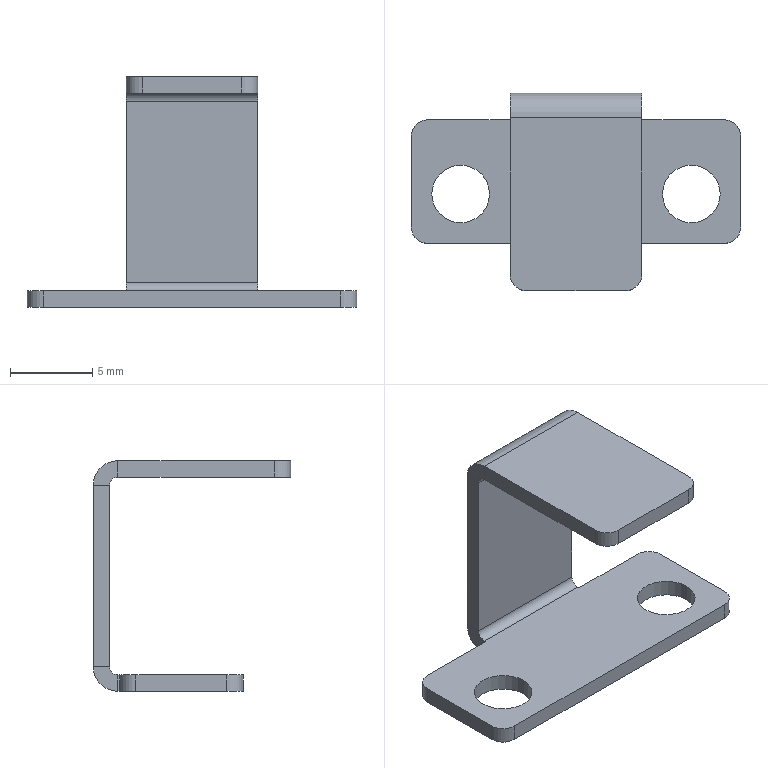Part | SolidWorks | features EdgeFlange 2, BreakCorner 1, FlatPattern 1, SMBaseFlange 1, SheetMetal 1 | 1 solid | 36 faces | box 20 x 12 x 14 mm | volume 327.403 mm3 | plane 22 | cylinder 14 | commonest cylinder face diameters 2 x6 3.5 x4 1 x2 3 x2
STEP:
#1=CARTESIAN_POINT('',(5.25,-0.75,-1.));
#2=VERTEX_POINT('',#1);
#3=CARTESIAN_POINT('',(8.75,-0.75,-1.));
#4=VERTEX_POINT('',#3);
#5=CARTESIAN_POINT('',(7.,-0.75,-1.));
#6=DIRECTION('',(0.,0.,1.));
#7=DIRECTION('',(1.,0.,0.));
#8=AXIS2_PLACEMENT_3D('',#5,#6,#7);
#9=CIRCLE('',#8,1.75);
#10=EDGE_CURVE('',#2,#4,#9,.T.);
#11=ORIENTED_EDGE('',*,*,#10,.F.);
#12=CARTESIAN_POINT('',(5.25,-0.75,0.));
#13=VERTEX_POINT('',#12);
#14=CARTESIAN_POINT('',(5.25,-0.75,-1.));
#15=DIRECTION('',(0.,0.,1.));
#16=VECTOR('',#15,1000.);
#17=LINE('',#14,#16);
#18=EDGE_CURVE('',#2,#13,#17,.T.);
#19=ORIENTED_EDGE('',*,*,#18,.T.);
#20=CARTESIAN_POINT('',(8.75,-0.75,0.));
#21=VERTEX_POINT('',#20);
#22=CARTESIAN_POINT('',(7.,-0.75,0.));
#23=DIRECTION('',(0.,0.,1.));
#24=DIRECTION('',(1.,0.,0.));
#25=AXIS2_PLACEMENT_3D('',#22,#23,#24);
#26=CIRCLE('',#25,1.75);
#27=EDGE_CURVE('',#13,#21,#26,.T.);
#28=ORIENTED_EDGE('',*,*,#27,.T.);
#29=CARTESIAN_POINT('',(8.75,-0.75,-1.));
#30=DIRECTION('',(0.,0.,1.));
#31=VECTOR('',#30,1000.);
#32=LINE('',#29,#31);
#33=EDGE_CURVE('',#4,#21,#32,.T.);
#34=ORIENTED_EDGE('',*,*,#33,.F.);
#35=EDGE_LOOP('',(#11,#19,#28,#34));
#36=FACE_OUTER_BOUND('',#35,.T.);
#37=CARTESIAN_POINT('',(7.,-0.75,-1.));
#38=DIRECTION('',(0.,0.,1.));
#39=DIRECTION('',(1.,0.,0.));
#40=AXIS2_PLACEMENT_3D('',#37,#38,#39);
#41=CYLINDRICAL_SURFACE('',#40,1.75);
#42=ADVANCED_FACE('',(#36),#41,.F.);
#43=CARTESIAN_POINT('',(-8.75,-0.75,-1.));
#44=VERTEX_POINT('',#43);
#45=CARTESIAN_POINT('',(-5.25,-0.75,-1.));
#46=VERTEX_POINT('',#45);
#47=CARTESIAN_POINT('',(-7.,-0.75,-1.));
#48=DIRECTION('',(0.,0.,1.));
#49=DIRECTION('',(1.,0.,0.));
#50=AXIS2_PLACEMENT_3D('',#47,#48,#49);
#51=CIRCLE('',#50,1.75);
#52=EDGE_CURVE('',#44,#46,#51,.T.);
#53=ORIENTED_EDGE('',*,*,#52,.F.);
#54=CARTESIAN_POINT('',(-8.75,-0.75,0.));
#55=VERTEX_POINT('',#54);
#56=CARTESIAN_POINT('',(-8.75,-0.75,-1.));
#57=DIRECTION('',(0.,0.,1.));
#58=VECTOR('',#57,1000.);
#59=LINE('',#56,#58);
#60=EDGE_CURVE('',#44,#55,#59,.T.);
#61=ORIENTED_EDGE('',*,*,#60,.T.);
#62=CARTESIAN_POINT('',(-5.25,-0.75,0.));
#63=VERTEX_POINT('',#62);
#64=CARTESIAN_POINT('',(-7.,-0.75,0.));
#65=DIRECTION('',(0.,0.,1.));
#66=DIRECTION('',(1.,0.,0.));
#67=AXIS2_PLACEMENT_3D('',#64,#65,#66);
#68=CIRCLE('',#67,1.75);
#69=EDGE_CURVE('',#55,#63,#68,.T.);
#70=ORIENTED_EDGE('',*,*,#69,.T.);
#71=CARTESIAN_POINT('',(-5.25,-0.75,-1.));
#72=DIRECTION('',(0.,0.,1.));
#73=VECTOR('',#72,1000.);
#74=LINE('',#71,#73);
#75=EDGE_CURVE('',#46,#63,#74,.T.);
#76=ORIENTED_EDGE('',*,*,#75,.F.);
#77=EDGE_LOOP('',(#53,#61,#70,#76));
#78=FACE_OUTER_BOUND('',#77,.T.);
#79=CARTESIAN_POINT('',(-7.,-0.75,-1.));
#80=DIRECTION('',(0.,0.,1.));
#81=DIRECTION('',(1.,0.,0.));
#82=AXIS2_PLACEMENT_3D('',#79,#80,#81);
#83=CYLINDRICAL_SURFACE('',#82,1.75);
#84=ADVANCED_FACE('',(#78),#83,.F.);
#85=CARTESIAN_POINT('',(4.,4.35,11.5));
#86=VERTEX_POINT('',#85);
#87=CARTESIAN_POINT('',(4.,5.35,11.5));
#88=VERTEX_POINT('',#87);
#89=CARTESIAN_POINT('',(4.,4.35,11.5));
#90=DIRECTION('',(0.,1.,0.));
#91=VECTOR('',#90,1000.);
#92=LINE('',#89,#91);
#93=EDGE_CURVE('',#86,#88,#92,.T.);
#94=ORIENTED_EDGE('',*,*,#93,.F.);
#95=CARTESIAN_POINT('',(4.,4.35,0.5));
#96=VERTEX_POINT('',#95);
#97=CARTESIAN_POINT('',(4.,4.35,0.));
#98=DIRECTION('',(0.,0.,-1.));
#99=VECTOR('',#98,1000.);
#100=LINE('',#97,#99);
#101=EDGE_CURVE('',#86,#96,#100,.T.);
#102=ORIENTED_EDGE('',*,*,#101,.T.);
#103=CARTESIAN_POINT('',(4.,5.35,0.5));
#104=VERTEX_POINT('',#103);
#105=CARTESIAN_POINT('',(4.,5.35,0.5));
#106=DIRECTION('',(0.,1.,0.));
#107=VECTOR('',#106,1000.);
#108=LINE('',#105,#107);
#109=EDGE_CURVE('',#96,#104,#108,.T.);
#110=ORIENTED_EDGE('',*,*,#109,.T.);
#111=CARTESIAN_POINT('',(4.,5.35,0.));
#112=DIRECTION('',(0.,0.,-1.));
#113=VECTOR('',#112,1000.);
#114=LINE('',#111,#113);
#115=EDGE_CURVE('',#88,#104,#114,.T.);
#116=ORIENTED_EDGE('',*,*,#115,.F.);
#117=EDGE_LOOP('',(#94,#102,#110,#116));
#118=FACE_OUTER_BOUND('',#117,.T.);
#119=CARTESIAN_POINT('',(4.,5.35,0.));
#120=DIRECTION('',(-1.,0.,0.));
#121=DIRECTION('',(0.,0.,1.));
#122=AXIS2_PLACEMENT_3D('',#119,#120,#121);
#123=PLANE('',#122);
#124=ADVANCED_FACE('',(#118),#123,.F.);
#125=CARTESIAN_POINT('',(-4.,4.35,11.5));
#126=VERTEX_POINT('',#125);
#127=CARTESIAN_POINT('',(-4.,5.35,11.5));
#128=VERTEX_POINT('',#127);
#129=CARTESIAN_POINT('',(-4.,4.35,11.5));
#130=DIRECTION('',(0.,1.,0.));
#131=VECTOR('',#130,1000.);
#132=LINE('',#129,#131);
#133=EDGE_CURVE('',#126,#128,#132,.T.);
#134=ORIENTED_EDGE('',*,*,#133,.T.);
#135=CARTESIAN_POINT('',(-4.,5.35,0.5));
#136=VERTEX_POINT('',#135);
#137=CARTESIAN_POINT('',(-4.,5.35,0.));
#138=DIRECTION('',(0.,0.,1.));
#139=VECTOR('',#138,1000.);
#140=LINE('',#137,#139);
#141=EDGE_CURVE('',#136,#128,#140,.T.);
#142=ORIENTED_EDGE('',*,*,#141,.F.);
#143=CARTESIAN_POINT('',(-4.,4.35,0.5));
#144=VERTEX_POINT('',#143);
#145=CARTESIAN_POINT('',(-4.,4.35,0.5));
#146=DIRECTION('',(0.,1.,0.));
#147=VECTOR('',#146,1000.);
#148=LINE('',#145,#147);
#149=EDGE_CURVE('',#144,#136,#148,.T.);
#150=ORIENTED_EDGE('',*,*,#149,.F.);
#151=CARTESIAN_POINT('',(-4.,4.35,13.));
#152=DIRECTION('',(0.,0.,1.));
#153=VECTOR('',#152,1000.);
#154=LINE('',#151,#153);
#155=EDGE_CURVE('',#144,#126,#154,.T.);
#156=ORIENTED_EDGE('',*,*,#155,.T.);
#157=EDGE_LOOP('',(#134,#142,#150,#156));
#158=FACE_OUTER_BOUND('',#157,.T.);
#159=CARTESIAN_POINT('',(-4.,5.35,13.));
#160=DIRECTION('',(1.,0.,0.));
#161=DIRECTION('',(0.,0.,-1.));
#162=AXIS2_PLACEMENT_3D('',#159,#160,#161);
#163=PLANE('',#162);
#164=ADVANCED_FACE('',(#158),#163,.F.);
#165=CARTESIAN_POINT('',(-4.,5.35,11.5));
#166=DIRECTION('',(1.,0.,0.));
#167=VECTOR('',#166,1000.);
#168=LINE('',#165,#167);
#169=EDGE_CURVE('',#128,#88,#168,.T.);
#170=ORIENTED_EDGE('',*,*,#169,.T.);
#171=ORIENTED_EDGE('',*,*,#115,.T.);
#172=CARTESIAN_POINT('',(4.,5.35,0.5));
#173=DIRECTION('',(1.,0.,0.));
#174=VECTOR('',#173,1000.);
#175=LINE('',#172,#174);
#176=EDGE_CURVE('',#136,#104,#175,.T.);
#177=ORIENTED_EDGE('',*,*,#176,.F.);
#178=ORIENTED_EDGE('',*,*,#141,.T.);
#179=EDGE_LOOP('',(#170,#171,#177,#178));
#180=FACE_OUTER_BOUND('',#179,.T.);
#181=CARTESIAN_POINT('',(0.,5.35,0.));
#182=DIRECTION('',(0.,-1.,0.));
#183=DIRECTION('',(0.,0.,-1.));
#184=AXIS2_PLACEMENT_3D('',#181,#182,#183);
#185=PLANE('',#184);
#186=ADVANCED_FACE('',(#180),#185,.F.);
#187=ORIENTED_EDGE('',*,*,#101,.F.);
#188=CARTESIAN_POINT('',(-4.,4.35,11.5));
#189=DIRECTION('',(1.,0.,0.));
#190=VECTOR('',#189,1000.);
#191=LINE('',#188,#190);
#192=EDGE_CURVE('',#126,#86,#191,.T.);
#193=ORIENTED_EDGE('',*,*,#192,.F.);
#194=ORIENTED_EDGE('',*,*,#155,.F.);
#195=CARTESIAN_POINT('',(4.,4.35,0.5));
#196=DIRECTION('',(-1.,0.,0.));
#197=VECTOR('',#196,1000.);
#198=LINE('',#195,#197);
#199=EDGE_CURVE('',#96,#144,#198,.T.);
#200=ORIENTED_EDGE('',*,*,#199,.F.);
#201=EDGE_LOOP('',(#187,#193,#194,#200));
#202=FACE_OUTER_BOUND('',#201,.T.);
#203=CARTESIAN_POINT('',(0.,4.35,0.));
#204=DIRECTION('',(0.,-1.,0.));
#205=DIRECTION('',(0.,0.,-1.));
#206=AXIS2_PLACEMENT_3D('',#203,#204,#205);
#207=PLANE('',#206);
#208=ADVANCED_FACE('',(#202),#207,.T.);
#209=CARTESIAN_POINT('',(-4.,3.75,-1.));
#210=VERTEX_POINT('',#209);
#211=CARTESIAN_POINT('',(-9.,3.75,-1.));
#212=VERTEX_POINT('',#211);
#213=CARTESIAN_POINT('',(-10.,3.75,-1.));
#214=DIRECTION('',(-1.,0.,0.));
#215=VECTOR('',#214,1000.);
#216=LINE('',#213,#215);
#217=EDGE_CURVE('',#210,#212,#216,.T.);
#218=ORIENTED_EDGE('',*,*,#217,.T.);
#219=CARTESIAN_POINT('',(-9.,3.75,0.));
#220=VERTEX_POINT('',#219);
#221=CARTESIAN_POINT('',(-9.,3.75,-1.));
#222=DIRECTION('',(0.,0.,1.));
#223=VECTOR('',#222,1000.);
#224=LINE('',#221,#223);
#225=EDGE_CURVE('',#212,#220,#224,.T.);
#226=ORIENTED_EDGE('',*,*,#225,.T.);
#227=CARTESIAN_POINT('',(-4.,3.75,0.));
#228=VERTEX_POINT('',#227);
#229=CARTESIAN_POINT('',(-10.,3.75,0.));
#230=DIRECTION('',(-1.,0.,0.));
#231=VECTOR('',#230,1000.);
#232=LINE('',#229,#231);
#233=EDGE_CURVE('',#228,#220,#232,.T.);
#234=ORIENTED_EDGE('',*,*,#233,.F.);
#235=CARTESIAN_POINT('',(-4.,3.75,0.));
#236=DIRECTION('',(0.,0.,-1.));
#237=VECTOR('',#236,1000.);
#238=LINE('',#235,#237);
#239=EDGE_CURVE('',#228,#210,#238,.T.);
#240=ORIENTED_EDGE('',*,*,#239,.T.);
#241=EDGE_LOOP('',(#218,#226,#234,#240));
#242=FACE_OUTER_BOUND('',#241,.T.);
#243=CARTESIAN_POINT('',(-10.,3.75,-1.));
#244=DIRECTION('',(0.,1.,0.));
#245=DIRECTION('',(0.,0.,1.));
#246=AXIS2_PLACEMENT_3D('',#243,#244,#245);
#247=PLANE('',#246);
#248=ADVANCED_FACE('',(#242),#247,.T.);
#249=CARTESIAN_POINT('',(10.,-2.75,0.));
#250=VERTEX_POINT('',#249);
#251=CARTESIAN_POINT('',(10.,2.75,0.));
#252=VERTEX_POINT('',#251);
#253=CARTESIAN_POINT('',(10.,-3.75,0.));
#254=DIRECTION('',(0.,1.,0.));
#255=VECTOR('',#254,1000.);
#256=LINE('',#253,#255);
#257=EDGE_CURVE('',#250,#252,#256,.T.);
#258=ORIENTED_EDGE('',*,*,#257,.F.);
#259=CARTESIAN_POINT('',(10.,-2.75,-1.));
#260=VERTEX_POINT('',#259);
#261=CARTESIAN_POINT('',(10.,-2.75,-1.));
#262=DIRECTION('',(0.,0.,-1.));
#263=VECTOR('',#262,1000.);
#264=LINE('',#261,#263);
#265=EDGE_CURVE('',#250,#260,#264,.T.);
#266=ORIENTED_EDGE('',*,*,#265,.T.);
#267=CARTESIAN_POINT('',(10.,2.75,-1.));
#268=VERTEX_POINT('',#267);
#269=CARTESIAN_POINT('',(10.,-3.75,-1.));
#270=DIRECTION('',(0.,1.,0.));
#271=VECTOR('',#270,1000.);
#272=LINE('',#269,#271);
#273=EDGE_CURVE('',#260,#268,#272,.T.);
#274=ORIENTED_EDGE('',*,*,#273,.T.);
#275=CARTESIAN_POINT('',(10.,2.75,-1.));
#276=DIRECTION('',(0.,0.,1.));
#277=VECTOR('',#276,1000.);
#278=LINE('',#275,#277);
#279=EDGE_CURVE('',#268,#252,#278,.T.);
#280=ORIENTED_EDGE('',*,*,#279,.T.);
#281=EDGE_LOOP('',(#258,#266,#274,#280));
#282=FACE_OUTER_BOUND('',#281,.T.);
#283=CARTESIAN_POINT('',(10.,-3.75,-1.));
#284=DIRECTION('',(1.,0.,0.));
#285=DIRECTION('',(0.,0.,-1.));
#286=AXIS2_PLACEMENT_3D('',#283,#284,#285);
#287=PLANE('',#286);
#288=ADVANCED_FACE('',(#282),#287,.T.);
#289=CARTESIAN_POINT('',(-9.,-3.75,-1.));
#290=VERTEX_POINT('',#289);
#291=CARTESIAN_POINT('',(9.,-3.75,-1.));
#292=VERTEX_POINT('',#291);
#293=CARTESIAN_POINT('',(-10.,-3.75,-1.));
#294=DIRECTION('',(1.,0.,0.));
#295=VECTOR('',#294,1000.);
#296=LINE('',#293,#295);
#297=EDGE_CURVE('',#290,#292,#296,.T.);
#298=ORIENTED_EDGE('',*,*,#297,.T.);
#299=CARTESIAN_POINT('',(9.,-3.75,0.));
#300=VERTEX_POINT('',#299);
#301=CARTESIAN_POINT('',(9.,-3.75,-1.));
#302=DIRECTION('',(0.,0.,1.));
#303=VECTOR('',#302,1000.);
#304=LINE('',#301,#303);
#305=EDGE_CURVE('',#292,#300,#304,.T.);
#306=ORIENTED_EDGE('',*,*,#305,.T.);
#307=CARTESIAN_POINT('',(-9.,-3.75,0.));
#308=VERTEX_POINT('',#307);
#309=CARTESIAN_POINT('',(-10.,-3.75,0.));
#310=DIRECTION('',(1.,0.,0.));
#311=VECTOR('',#310,1000.);
#312=LINE('',#309,#311);
#313=EDGE_CURVE('',#308,#300,#312,.T.);
#314=ORIENTED_EDGE('',*,*,#313,.F.);
#315=CARTESIAN_POINT('',(-9.,-3.75,-1.));
#316=DIRECTION('',(0.,0.,-1.));
#317=VECTOR('',#316,1000.);
#318=LINE('',#315,#317);
#319=EDGE_CURVE('',#308,#290,#318,.T.);
#320=ORIENTED_EDGE('',*,*,#319,.T.);
#321=EDGE_LOOP('',(#298,#306,#314,#320));
#322=FACE_OUTER_BOUND('',#321,.T.);
#323=CARTESIAN_POINT('',(-10.,-3.75,-1.));
#324=DIRECTION('',(0.,-1.,0.));
#325=DIRECTION('',(0.,0.,-1.));
#326=AXIS2_PLACEMENT_3D('',#323,#324,#325);
#327=PLANE('',#326);
#328=ADVANCED_FACE('',(#322),#327,.T.);
#329=CARTESIAN_POINT('',(-10.,2.75,-1.));
#330=VERTEX_POINT('',#329);
#331=CARTESIAN_POINT('',(-10.,-2.75,-1.));
#332=VERTEX_POINT('',#331);
#333=CARTESIAN_POINT('',(-10.,-3.75,-1.));
#334=DIRECTION('',(0.,-1.,0.));
#335=VECTOR('',#334,1000.);
#336=LINE('',#333,#335);
#337=EDGE_CURVE('',#330,#332,#336,.T.);
#338=ORIENTED_EDGE('',*,*,#337,.T.);
#339=CARTESIAN_POINT('',(-10.,-2.75,0.));
#340=VERTEX_POINT('',#339);
#341=CARTESIAN_POINT('',(-10.,-2.75,-1.));
#342=DIRECTION('',(0.,0.,1.));
#343=VECTOR('',#342,1000.);
#344=LINE('',#341,#343);
#345=EDGE_CURVE('',#332,#340,#344,.T.);
#346=ORIENTED_EDGE('',*,*,#345,.T.);
#347=CARTESIAN_POINT('',(-10.,2.75,0.));
#348=VERTEX_POINT('',#347);
#349=CARTESIAN_POINT('',(-10.,-3.75,0.));
#350=DIRECTION('',(0.,-1.,0.));
#351=VECTOR('',#350,1000.);
#352=LINE('',#349,#351);
#353=EDGE_CURVE('',#348,#340,#352,.T.);
#354=ORIENTED_EDGE('',*,*,#353,.F.);
#355=CARTESIAN_POINT('',(-10.,2.75,-1.));
#356=DIRECTION('',(0.,0.,-1.));
#357=VECTOR('',#356,1000.);
#358=LINE('',#355,#357);
#359=EDGE_CURVE('',#348,#330,#358,.T.);
#360=ORIENTED_EDGE('',*,*,#359,.T.);
#361=EDGE_LOOP('',(#338,#346,#354,#360));
#362=FACE_OUTER_BOUND('',#361,.T.);
#363=CARTESIAN_POINT('',(-10.,-3.75,-1.));
#364=DIRECTION('',(-1.,0.,0.));
#365=DIRECTION('',(0.,0.,1.));
#366=AXIS2_PLACEMENT_3D('',#363,#364,#365);
#367=PLANE('',#366);
#368=ADVANCED_FACE('',(#362),#367,.T.);
#369=CARTESIAN_POINT('',(9.,3.75,0.));
#370=VERTEX_POINT('',#369);
#371=CARTESIAN_POINT('',(4.,3.75,0.));
#372=VERTEX_POINT('',#371);
#373=CARTESIAN_POINT('',(-10.,3.75,0.));
#374=DIRECTION('',(-1.,0.,0.));
#375=VECTOR('',#374,1000.);
#376=LINE('',#373,#375);
#377=EDGE_CURVE('',#370,#372,#376,.T.);
#378=ORIENTED_EDGE('',*,*,#377,.F.);
#379=CARTESIAN_POINT('',(9.,3.75,-1.));
#380=VERTEX_POINT('',#379);
#381=CARTESIAN_POINT('',(9.,3.75,-1.));
#382=DIRECTION('',(0.,0.,-1.));
#383=VECTOR('',#382,1000.);
#384=LINE('',#381,#383);
#385=EDGE_CURVE('',#370,#380,#384,.T.);
#386=ORIENTED_EDGE('',*,*,#385,.T.);
#387=CARTESIAN_POINT('',(4.,3.75,-1.));
#388=VERTEX_POINT('',#387);
#389=CARTESIAN_POINT('',(-10.,3.75,-1.));
#390=DIRECTION('',(-1.,0.,0.));
#391=VECTOR('',#390,1000.);
#392=LINE('',#389,#391);
#393=EDGE_CURVE('',#380,#388,#392,.T.);
#394=ORIENTED_EDGE('',*,*,#393,.T.);
#395=CARTESIAN_POINT('',(4.,3.75,0.));
#396=DIRECTION('',(0.,0.,-1.));
#397=VECTOR('',#396,1000.);
#398=LINE('',#395,#397);
#399=EDGE_CURVE('',#372,#388,#398,.T.);
#400=ORIENTED_EDGE('',*,*,#399,.F.);
#401=EDGE_LOOP('',(#378,#386,#394,#400));
#402=FACE_OUTER_BOUND('',#401,.T.);
#403=CARTESIAN_POINT('',(-10.,3.75,-1.));
#404=DIRECTION('',(0.,1.,0.));
#405=DIRECTION('',(0.,0.,1.));
#406=AXIS2_PLACEMENT_3D('',#403,#404,#405);
#407=PLANE('',#406);
#408=ADVANCED_FACE('',(#402),#407,.T.);
#409=CARTESIAN_POINT('',(7.,-0.75,-1.));
#410=DIRECTION('',(0.,0.,1.));
#411=DIRECTION('',(1.,0.,0.));
#412=AXIS2_PLACEMENT_3D('',#409,#410,#411);
#413=CIRCLE('',#412,1.75);
#414=EDGE_CURVE('',#4,#2,#413,.T.);
#415=ORIENTED_EDGE('',*,*,#414,.T.);
#416=ORIENTED_EDGE('',*,*,#10,.T.);
#417=EDGE_LOOP('',(#415,#416));
#418=FACE_BOUND('',#417,.T.);
#419=CARTESIAN_POINT('',(-7.,-0.75,-1.));
#420=DIRECTION('',(0.,0.,1.));
#421=DIRECTION('',(1.,0.,0.));
#422=AXIS2_PLACEMENT_3D('',#419,#420,#421);
#423=CIRCLE('',#422,1.75);
#424=EDGE_CURVE('',#46,#44,#423,.T.);
#425=ORIENTED_EDGE('',*,*,#424,.T.);
#426=ORIENTED_EDGE('',*,*,#52,.T.);
#427=EDGE_LOOP('',(#425,#426));
#428=FACE_BOUND('',#427,.T.);
#429=ORIENTED_EDGE('',*,*,#273,.F.);
#430=CARTESIAN_POINT('',(9.,-2.75,-1.));
#431=DIRECTION('',(0.,0.,-1.));
#432=DIRECTION('',(-1.,0.,0.));
#433=AXIS2_PLACEMENT_3D('',#430,#431,#432);
#434=CIRCLE('',#433,1.);
#435=EDGE_CURVE('',#260,#292,#434,.T.);
#436=ORIENTED_EDGE('',*,*,#435,.T.);
#437=ORIENTED_EDGE('',*,*,#297,.F.);
#438=CARTESIAN_POINT('',(-9.,-2.75,-1.));
#439=DIRECTION('',(0.,0.,-1.));
#440=DIRECTION('',(-1.,0.,0.));
#441=AXIS2_PLACEMENT_3D('',#438,#439,#440);
#442=CIRCLE('',#441,1.);
#443=EDGE_CURVE('',#290,#332,#442,.T.);
#444=ORIENTED_EDGE('',*,*,#443,.T.);
#445=ORIENTED_EDGE('',*,*,#337,.F.);
#446=CARTESIAN_POINT('',(-9.,2.75,-1.));
#447=DIRECTION('',(0.,0.,-1.));
#448=DIRECTION('',(-1.,0.,0.));
#449=AXIS2_PLACEMENT_3D('',#446,#447,#448);
#450=CIRCLE('',#449,1.);
#451=EDGE_CURVE('',#330,#212,#450,.T.);
#452=ORIENTED_EDGE('',*,*,#451,.T.);
#453=ORIENTED_EDGE('',*,*,#217,.F.);
#454=CARTESIAN_POINT('',(-4.,3.85,-1.));
#455=VERTEX_POINT('',#454);
#456=CARTESIAN_POINT('',(-4.,3.85,-1.));
#457=DIRECTION('',(0.,-1.,0.));
#458=VECTOR('',#457,1000.);
#459=LINE('',#456,#458);
#460=EDGE_CURVE('',#455,#210,#459,.T.);
#461=ORIENTED_EDGE('',*,*,#460,.F.);
#462=CARTESIAN_POINT('',(4.,3.85,-1.));
#463=VERTEX_POINT('',#462);
#464=CARTESIAN_POINT('',(-4.,3.85,-1.));
#465=DIRECTION('',(1.,0.,0.));
#466=VECTOR('',#465,1000.);
#467=LINE('',#464,#466);
#468=EDGE_CURVE('',#455,#463,#467,.T.);
#469=ORIENTED_EDGE('',*,*,#468,.T.);
#470=CARTESIAN_POINT('',(4.,3.85,-1.));
#471=DIRECTION('',(0.,-1.,0.));
#472=VECTOR('',#471,1000.);
#473=LINE('',#470,#472);
#474=EDGE_CURVE('',#463,#388,#473,.T.);
#475=ORIENTED_EDGE('',*,*,#474,.T.);
#476=ORIENTED_EDGE('',*,*,#393,.F.);
#477=CARTESIAN_POINT('',(9.,2.75,-1.));
#478=DIRECTION('',(0.,0.,-1.));
#479=DIRECTION('',(-1.,0.,0.));
#480=AXIS2_PLACEMENT_3D('',#477,#478,#479);
#481=CIRCLE('',#480,1.);
#482=EDGE_CURVE('',#380,#268,#481,.T.);
#483=ORIENTED_EDGE('',*,*,#482,.T.);
#484=EDGE_LOOP('',(#429,#436,#437,#444,#445,#452,#453,#461,#469,#475,#476,#483));
#485=FACE_OUTER_BOUND('',#484,.T.);
#486=CARTESIAN_POINT('',(0.,0.,-1.));
#487=DIRECTION('',(0.,0.,-1.));
#488=DIRECTION('',(-1.,0.,0.));
#489=AXIS2_PLACEMENT_3D('',#486,#487,#488);
#490=PLANE('',#489);
#491=ADVANCED_FACE('',(#418,#428,#485),#490,.T.);
#492=CARTESIAN_POINT('',(7.,-0.75,0.));
#493=DIRECTION('',(0.,0.,1.));
#494=DIRECTION('',(1.,0.,0.));
#495=AXIS2_PLACEMENT_3D('',#492,#493,#494);
#496=CIRCLE('',#495,1.75);
#497=EDGE_CURVE('',#21,#13,#496,.T.);
#498=ORIENTED_EDGE('',*,*,#497,.F.);
#499=ORIENTED_EDGE('',*,*,#27,.F.);
#500=EDGE_LOOP('',(#498,#499));
#501=FACE_BOUND('',#500,.T.);
#502=CARTESIAN_POINT('',(-7.,-0.75,0.));
#503=DIRECTION('',(0.,0.,1.));
#504=DIRECTION('',(1.,0.,0.));
#505=AXIS2_PLACEMENT_3D('',#502,#503,#504);
#506=CIRCLE('',#505,1.75);
#507=EDGE_CURVE('',#63,#55,#506,.T.);
#508=ORIENTED_EDGE('',*,*,#507,.F.);
#509=ORIENTED_EDGE('',*,*,#69,.F.);
#510=EDGE_LOOP('',(#508,#509));
#511=FACE_BOUND('',#510,.T.);
#512=ORIENTED_EDGE('',*,*,#313,.T.);
#513=CARTESIAN_POINT('',(9.,-2.75,0.));
#514=DIRECTION('',(0.,0.,1.));
#515=DIRECTION('',(-1.,0.,0.));
#516=AXIS2_PLACEMENT_3D('',#513,#514,#515);
#517=CIRCLE('',#516,1.);
#518=EDGE_CURVE('',#300,#250,#517,.T.);
#519=ORIENTED_EDGE('',*,*,#518,.T.);
#520=ORIENTED_EDGE('',*,*,#257,.T.);
#521=CARTESIAN_POINT('',(9.,2.75,0.));
#522=DIRECTION('',(0.,0.,1.));
#523=DIRECTION('',(-1.,0.,0.));
#524=AXIS2_PLACEMENT_3D('',#521,#522,#523);
#525=CIRCLE('',#524,1.);
#526=EDGE_CURVE('',#252,#370,#525,.T.);
#527=ORIENTED_EDGE('',*,*,#526,.T.);
#528=ORIENTED_EDGE('',*,*,#377,.T.);
#529=CARTESIAN_POINT('',(4.,3.85,0.));
#530=VERTEX_POINT('',#529);
#531=CARTESIAN_POINT('',(4.,3.85,0.));
#532=DIRECTION('',(0.,-1.,0.));
#533=VECTOR('',#532,1000.);
#534=LINE('',#531,#533);
#535=EDGE_CURVE('',#530,#372,#534,.T.);
#536=ORIENTED_EDGE('',*,*,#535,.F.);
#537=CARTESIAN_POINT('',(-4.,3.85,0.));
#538=VERTEX_POINT('',#537);
#539=CARTESIAN_POINT('',(-4.,3.85,0.));
#540=DIRECTION('',(1.,0.,0.));
#541=VECTOR('',#540,1000.);
#542=LINE('',#539,#541);
#543=EDGE_CURVE('',#538,#530,#542,.T.);
#544=ORIENTED_EDGE('',*,*,#543,.F.);
#545=CARTESIAN_POINT('',(-4.,3.85,0.));
#546=DIRECTION('',(0.,-1.,0.));
#547=VECTOR('',#546,1000.);
#548=LINE('',#545,#547);
#549=EDGE_CURVE('',#538,#228,#548,.T.);
#550=ORIENTED_EDGE('',*,*,#549,.T.);
#551=ORIENTED_EDGE('',*,*,#233,.T.);
#552=CARTESIAN_POINT('',(-9.,2.75,0.));
#553=DIRECTION('',(0.,0.,1.));
#554=DIRECTION('',(-1.,0.,0.));
#555=AXIS2_PLACEMENT_3D('',#552,#553,#554);
#556=CIRCLE('',#555,1.);
#557=EDGE_CURVE('',#220,#348,#556,.T.);
#558=ORIENTED_EDGE('',*,*,#557,.T.);
#559=ORIENTED_EDGE('',*,*,#353,.T.);
#560=CARTESIAN_POINT('',(-9.,-2.75,0.));
#561=DIRECTION('',(0.,0.,1.));
#562=DIRECTION('',(-1.,0.,0.));
#563=AXIS2_PLACEMENT_3D('',#560,#561,#562);
#564=CIRCLE('',#563,1.);
#565=EDGE_CURVE('',#340,#308,#564,.T.);
#566=ORIENTED_EDGE('',*,*,#565,.T.);
#567=EDGE_LOOP('',(#512,#519,#520,#527,#528,#536,#544,#550,#551,#558,#559,#566));
#568=FACE_OUTER_BOUND('',#567,.T.);
#569=CARTESIAN_POINT('',(0.,0.,0.));
#570=DIRECTION('',(0.,0.,-1.));
#571=DIRECTION('',(-1.,0.,0.));
#572=AXIS2_PLACEMENT_3D('',#569,#570,#571);
#573=PLANE('',#572);
#574=ADVANCED_FACE('',(#501,#511,#568),#573,.F.);
#575=ORIENTED_EDGE('',*,*,#60,.F.);
#576=ORIENTED_EDGE('',*,*,#424,.F.);
#577=ORIENTED_EDGE('',*,*,#75,.T.);
#578=ORIENTED_EDGE('',*,*,#507,.T.);
#579=EDGE_LOOP('',(#575,#576,#577,#578));
#580=FACE_OUTER_BOUND('',#579,.T.);
#581=CARTESIAN_POINT('',(-7.,-0.75,-1.));
#582=DIRECTION('',(0.,0.,1.));
#583=DIRECTION('',(1.,0.,0.));
#584=AXIS2_PLACEMENT_3D('',#581,#582,#583);
#585=CYLINDRICAL_SURFACE('',#584,1.75);
#586=ADVANCED_FACE('',(#580),#585,.F.);
#587=ORIENTED_EDGE('',*,*,#18,.F.);
#588=ORIENTED_EDGE('',*,*,#414,.F.);
#589=ORIENTED_EDGE('',*,*,#33,.T.);
#590=ORIENTED_EDGE('',*,*,#497,.T.);
#591=EDGE_LOOP('',(#587,#588,#589,#590));
#592=FACE_OUTER_BOUND('',#591,.T.);
#593=CARTESIAN_POINT('',(7.,-0.75,-1.));
#594=DIRECTION('',(0.,0.,1.));
#595=DIRECTION('',(1.,0.,0.));
#596=AXIS2_PLACEMENT_3D('',#593,#594,#595);
#597=CYLINDRICAL_SURFACE('',#596,1.75);
#598=ADVANCED_FACE('',(#592),#597,.F.);
#599=ORIENTED_EDGE('',*,*,#549,.F.);
#600=CARTESIAN_POINT('',(-4.,3.85,0.));
#601=DIRECTION('',(0.,0.,-1.));
#602=VECTOR('',#601,1000.);
#603=LINE('',#600,#602);
#604=EDGE_CURVE('',#538,#455,#603,.T.);
#605=ORIENTED_EDGE('',*,*,#604,.T.);
#606=ORIENTED_EDGE('',*,*,#460,.T.);
#607=ORIENTED_EDGE('',*,*,#239,.F.);
#608=EDGE_LOOP('',(#599,#605,#606,#607));
#609=FACE_OUTER_BOUND('',#608,.T.);
#610=CARTESIAN_POINT('',(-4.,3.85,0.));
#611=DIRECTION('',(-1.,0.,0.));
#612=DIRECTION('',(0.,0.,-1.));
#613=AXIS2_PLACEMENT_3D('',#610,#611,#612);
#614=PLANE('',#613);
#615=ADVANCED_FACE('',(#609),#614,.T.);
#616=ORIENTED_EDGE('',*,*,#474,.F.);
#617=CARTESIAN_POINT('',(4.,3.85,0.));
#618=DIRECTION('',(0.,0.,-1.));
#619=VECTOR('',#618,1000.);
#620=LINE('',#617,#619);
#621=EDGE_CURVE('',#530,#463,#620,.T.);
#622=ORIENTED_EDGE('',*,*,#621,.F.);
#623=ORIENTED_EDGE('',*,*,#535,.T.);
#624=ORIENTED_EDGE('',*,*,#399,.T.);
#625=EDGE_LOOP('',(#616,#622,#623,#624));
#626=FACE_OUTER_BOUND('',#625,.T.);
#627=CARTESIAN_POINT('',(4.,3.85,0.));
#628=DIRECTION('',(-1.,0.,0.));
#629=DIRECTION('',(0.,0.,-1.));
#630=AXIS2_PLACEMENT_3D('',#627,#628,#629);
#631=PLANE('',#630);
#632=ADVANCED_FACE('',(#626),#631,.F.);
#633=ORIENTED_EDGE('',*,*,#109,.F.);
#634=CARTESIAN_POINT('',(4.,3.85,0.5));
#635=DIRECTION('',(1.,0.,0.));
#636=DIRECTION('',(0.,0.,1.));
#637=AXIS2_PLACEMENT_3D('',#634,#635,#636);
#638=CIRCLE('',#637,0.5);
#639=EDGE_CURVE('',#530,#96,#638,.T.);
#640=ORIENTED_EDGE('',*,*,#639,.F.);
#641=ORIENTED_EDGE('',*,*,#621,.T.);
#642=CARTESIAN_POINT('',(4.,3.85,0.5));
#643=DIRECTION('',(1.,0.,0.));
#644=DIRECTION('',(0.,0.,1.));
#645=AXIS2_PLACEMENT_3D('',#642,#643,#644);
#646=CIRCLE('',#645,1.5);
#647=EDGE_CURVE('',#463,#104,#646,.T.);
#648=ORIENTED_EDGE('',*,*,#647,.T.);
#649=EDGE_LOOP('',(#633,#640,#641,#648));
#650=FACE_OUTER_BOUND('',#649,.T.);
#651=CARTESIAN_POINT('',(4.,3.85,0.5));
#652=DIRECTION('',(1.,0.,0.));
#653=DIRECTION('',(0.,0.,-1.));
#654=AXIS2_PLACEMENT_3D('',#651,#652,#653);
#655=PLANE('',#654);
#656=ADVANCED_FACE('',(#650),#655,.T.);
#657=CARTESIAN_POINT('',(-4.,3.85,0.5));
#658=DIRECTION('',(-1.,0.,0.));
#659=DIRECTION('',(0.,0.,1.));
#660=AXIS2_PLACEMENT_3D('',#657,#658,#659);
#661=CIRCLE('',#660,0.5);
#662=EDGE_CURVE('',#144,#538,#661,.T.);
#663=ORIENTED_EDGE('',*,*,#662,.F.);
#664=ORIENTED_EDGE('',*,*,#149,.T.);
#665=CARTESIAN_POINT('',(-4.,3.85,0.5));
#666=DIRECTION('',(-1.,0.,0.));
#667=DIRECTION('',(0.,0.,1.));
#668=AXIS2_PLACEMENT_3D('',#665,#666,#667);
#669=CIRCLE('',#668,1.5);
#670=EDGE_CURVE('',#136,#455,#669,.T.);
#671=ORIENTED_EDGE('',*,*,#670,.T.);
#672=ORIENTED_EDGE('',*,*,#604,.F.);
#673=EDGE_LOOP('',(#663,#664,#671,#672));
#674=FACE_OUTER_BOUND('',#673,.T.);
#675=CARTESIAN_POINT('',(-4.,3.85,0.5));
#676=DIRECTION('',(1.,0.,0.));
#677=DIRECTION('',(0.,0.,-1.));
#678=AXIS2_PLACEMENT_3D('',#675,#676,#677);
#679=PLANE('',#678);
#680=ADVANCED_FACE('',(#674),#679,.F.);
#681=ORIENTED_EDGE('',*,*,#468,.F.);
#682=ORIENTED_EDGE('',*,*,#670,.F.);
#683=ORIENTED_EDGE('',*,*,#176,.T.);
#684=ORIENTED_EDGE('',*,*,#647,.F.);
#685=EDGE_LOOP('',(#681,#682,#683,#684));
#686=FACE_OUTER_BOUND('',#685,.T.);
#687=CARTESIAN_POINT('',(-4.,3.85,0.5));
#688=DIRECTION('',(-1.,0.,0.));
#689=DIRECTION('',(0.,1.,0.));
#690=AXIS2_PLACEMENT_3D('',#687,#688,#689);
#691=CYLINDRICAL_SURFACE('',#690,1.5);
#692=ADVANCED_FACE('',(#686),#691,.T.);
#693=ORIENTED_EDGE('',*,*,#543,.T.);
#694=ORIENTED_EDGE('',*,*,#639,.T.);
#695=ORIENTED_EDGE('',*,*,#199,.T.);
#696=ORIENTED_EDGE('',*,*,#662,.T.);
#697=EDGE_LOOP('',(#693,#694,#695,#696));
#698=FACE_OUTER_BOUND('',#697,.T.);
#699=CARTESIAN_POINT('',(-4.,3.85,0.5));
#700=DIRECTION('',(-1.,0.,0.));
#701=DIRECTION('',(0.,1.,0.));
#702=AXIS2_PLACEMENT_3D('',#699,#700,#701);
#703=CYLINDRICAL_SURFACE('',#702,0.5);
#704=ADVANCED_FACE('',(#698),#703,.F.);
#705=CARTESIAN_POINT('',(4.,3.85,12.));
#706=VERTEX_POINT('',#705);
#707=CARTESIAN_POINT('',(4.,3.85,13.));
#708=VERTEX_POINT('',#707);
#709=CARTESIAN_POINT('',(4.,3.85,13.));
#710=DIRECTION('',(0.,0.,1.));
#711=VECTOR('',#710,1000.);
#712=LINE('',#709,#711);
#713=EDGE_CURVE('',#706,#708,#712,.T.);
#714=ORIENTED_EDGE('',*,*,#713,.F.);
#715=CARTESIAN_POINT('',(4.,3.85,11.5));
#716=DIRECTION('',(1.,0.,0.));
#717=DIRECTION('',(0.,0.,1.));
#718=AXIS2_PLACEMENT_3D('',#715,#716,#717);
#719=CIRCLE('',#718,0.5);
#720=EDGE_CURVE('',#86,#706,#719,.T.);
#721=ORIENTED_EDGE('',*,*,#720,.F.);
#722=ORIENTED_EDGE('',*,*,#93,.T.);
#723=CARTESIAN_POINT('',(4.,3.85,11.5));
#724=DIRECTION('',(1.,0.,0.));
#725=DIRECTION('',(0.,0.,1.));
#726=AXIS2_PLACEMENT_3D('',#723,#724,#725);
#727=CIRCLE('',#726,1.5);
#728=EDGE_CURVE('',#88,#708,#727,.T.);
#729=ORIENTED_EDGE('',*,*,#728,.T.);
#730=EDGE_LOOP('',(#714,#721,#722,#729));
#731=FACE_OUTER_BOUND('',#730,.T.);
#732=CARTESIAN_POINT('',(4.,3.85,11.5));
#733=DIRECTION('',(1.,0.,0.));
#734=DIRECTION('',(0.,0.,-1.));
#735=AXIS2_PLACEMENT_3D('',#732,#733,#734);
#736=PLANE('',#735);
#737=ADVANCED_FACE('',(#731),#736,.T.);
#738=CARTESIAN_POINT('',(-4.,3.85,12.));
#739=VERTEX_POINT('',#738);
#740=CARTESIAN_POINT('',(-4.,3.85,11.5));
#741=DIRECTION('',(-1.,0.,0.));
#742=DIRECTION('',(0.,0.,1.));
#743=AXIS2_PLACEMENT_3D('',#740,#741,#742);
#744=CIRCLE('',#743,0.5);
#745=EDGE_CURVE('',#739,#126,#744,.T.);
#746=ORIENTED_EDGE('',*,*,#745,.F.);
#747=CARTESIAN_POINT('',(-4.,3.85,13.));
#748=VERTEX_POINT('',#747);
#749=CARTESIAN_POINT('',(-4.,3.85,12.));
#750=DIRECTION('',(0.,0.,1.));
#751=VECTOR('',#750,1000.);
#752=LINE('',#749,#751);
#753=EDGE_CURVE('',#739,#748,#752,.T.);
#754=ORIENTED_EDGE('',*,*,#753,.T.);
#755=CARTESIAN_POINT('',(-4.,3.85,11.5));
#756=DIRECTION('',(-1.,0.,0.));
#757=DIRECTION('',(0.,0.,1.));
#758=AXIS2_PLACEMENT_3D('',#755,#756,#757);
#759=CIRCLE('',#758,1.5);
#760=EDGE_CURVE('',#748,#128,#759,.T.);
#761=ORIENTED_EDGE('',*,*,#760,.T.);
#762=ORIENTED_EDGE('',*,*,#133,.F.);
#763=EDGE_LOOP('',(#746,#754,#761,#762));
#764=FACE_OUTER_BOUND('',#763,.T.);
#765=CARTESIAN_POINT('',(-4.,3.85,11.5));
#766=DIRECTION('',(1.,0.,0.));
#767=DIRECTION('',(0.,0.,-1.));
#768=AXIS2_PLACEMENT_3D('',#765,#766,#767);
#769=PLANE('',#768);
#770=ADVANCED_FACE('',(#764),#769,.F.);
#771=ORIENTED_EDGE('',*,*,#169,.F.);
#772=ORIENTED_EDGE('',*,*,#760,.F.);
#773=CARTESIAN_POINT('',(4.,3.85,13.));
#774=DIRECTION('',(1.,0.,0.));
#775=VECTOR('',#774,1000.);
#776=LINE('',#773,#775);
#777=EDGE_CURVE('',#748,#708,#776,.T.);
#778=ORIENTED_EDGE('',*,*,#777,.T.);
#779=ORIENTED_EDGE('',*,*,#728,.F.);
#780=EDGE_LOOP('',(#771,#772,#778,#779));
#781=FACE_OUTER_BOUND('',#780,.T.);
#782=CARTESIAN_POINT('',(-4.,3.85,11.5));
#783=DIRECTION('',(-1.,0.,0.));
#784=DIRECTION('',(0.,0.,1.));
#785=AXIS2_PLACEMENT_3D('',#782,#783,#784);
#786=CYLINDRICAL_SURFACE('',#785,1.5);
#787=ADVANCED_FACE('',(#781),#786,.T.);
#788=ORIENTED_EDGE('',*,*,#192,.T.);
#789=ORIENTED_EDGE('',*,*,#720,.T.);
#790=CARTESIAN_POINT('',(4.,3.85,12.));
#791=DIRECTION('',(-1.,0.,0.));
#792=VECTOR('',#791,1000.);
#793=LINE('',#790,#792);
#794=EDGE_CURVE('',#706,#739,#793,.T.);
#795=ORIENTED_EDGE('',*,*,#794,.T.);
#796=ORIENTED_EDGE('',*,*,#745,.T.);
#797=EDGE_LOOP('',(#788,#789,#795,#796));
#798=FACE_OUTER_BOUND('',#797,.T.);
#799=CARTESIAN_POINT('',(-4.,3.85,11.5));
#800=DIRECTION('',(-1.,0.,0.));
#801=DIRECTION('',(0.,0.,1.));
#802=AXIS2_PLACEMENT_3D('',#799,#800,#801);
#803=CYLINDRICAL_SURFACE('',#802,0.5);
#804=ADVANCED_FACE('',(#798),#803,.F.);
#805=CARTESIAN_POINT('',(-4.,-5.65,12.));
#806=VERTEX_POINT('',#805);
#807=CARTESIAN_POINT('',(-4.,-6.65,12.));
#808=DIRECTION('',(0.,-1.,0.));
#809=VECTOR('',#808,1000.);
#810=LINE('',#807,#809);
#811=EDGE_CURVE('',#739,#806,#810,.T.);
#812=ORIENTED_EDGE('',*,*,#811,.T.);
#813=CARTESIAN_POINT('',(-4.,-5.65,13.));
#814=VERTEX_POINT('',#813);
#815=CARTESIAN_POINT('',(-4.,-5.65,13.));
#816=DIRECTION('',(0.,0.,1.));
#817=VECTOR('',#816,1000.);
#818=LINE('',#815,#817);
#819=EDGE_CURVE('',#806,#814,#818,.T.);
#820=ORIENTED_EDGE('',*,*,#819,.T.);
#821=CARTESIAN_POINT('',(-4.,0.,13.));
#822=DIRECTION('',(0.,-1.,0.));
#823=VECTOR('',#822,1000.);
#824=LINE('',#821,#823);
#825=EDGE_CURVE('',#748,#814,#824,.T.);
#826=ORIENTED_EDGE('',*,*,#825,.F.);
#827=ORIENTED_EDGE('',*,*,#753,.F.);
#828=EDGE_LOOP('',(#812,#820,#826,#827));
#829=FACE_OUTER_BOUND('',#828,.T.);
#830=CARTESIAN_POINT('',(-4.,-6.65,13.));
#831=DIRECTION('',(1.,0.,0.));
#832=DIRECTION('',(0.,0.,-1.));
#833=AXIS2_PLACEMENT_3D('',#830,#831,#832);
#834=PLANE('',#833);
#835=ADVANCED_FACE('',(#829),#834,.F.);
#836=CARTESIAN_POINT('',(4.,-5.65,13.));
#837=VERTEX_POINT('',#836);
#838=CARTESIAN_POINT('',(4.,0.,13.));
#839=DIRECTION('',(0.,1.,0.));
#840=VECTOR('',#839,1000.);
#841=LINE('',#838,#840);
#842=EDGE_CURVE('',#837,#708,#841,.T.);
#843=ORIENTED_EDGE('',*,*,#842,.F.);
#844=CARTESIAN_POINT('',(4.,-5.65,12.));
#845=VERTEX_POINT('',#844);
#846=CARTESIAN_POINT('',(4.,-5.65,13.));
#847=DIRECTION('',(0.,0.,-1.));
#848=VECTOR('',#847,1000.);
#849=LINE('',#846,#848);
#850=EDGE_CURVE('',#837,#845,#849,.T.);
#851=ORIENTED_EDGE('',*,*,#850,.T.);
#852=CARTESIAN_POINT('',(4.,4.35,12.));
#853=DIRECTION('',(0.,1.,0.));
#854=VECTOR('',#853,1000.);
#855=LINE('',#852,#854);
#856=EDGE_CURVE('',#845,#706,#855,.T.);
#857=ORIENTED_EDGE('',*,*,#856,.T.);
#858=ORIENTED_EDGE('',*,*,#713,.T.);
#859=EDGE_LOOP('',(#843,#851,#857,#858));
#860=FACE_OUTER_BOUND('',#859,.T.);
#861=CARTESIAN_POINT('',(4.,4.35,13.));
#862=DIRECTION('',(-1.,0.,0.));
#863=DIRECTION('',(0.,0.,1.));
#864=AXIS2_PLACEMENT_3D('',#861,#862,#863);
#865=PLANE('',#864);
#866=ADVANCED_FACE('',(#860),#865,.F.);
#867=ORIENTED_EDGE('',*,*,#825,.T.);
#868=CARTESIAN_POINT('',(-3.,-6.65,13.));
#869=VERTEX_POINT('',#868);
#870=CARTESIAN_POINT('',(-3.,-5.65,13.));
#871=DIRECTION('',(0.,0.,1.));
#872=DIRECTION('',(0.,1.,0.));
#873=AXIS2_PLACEMENT_3D('',#870,#871,#872);
#874=CIRCLE('',#873,1.);
#875=EDGE_CURVE('',#814,#869,#874,.T.);
#876=ORIENTED_EDGE('',*,*,#875,.T.);
#877=CARTESIAN_POINT('',(3.,-6.65,13.));
#878=VERTEX_POINT('',#877);
#879=CARTESIAN_POINT('',(0.,-6.65,13.));
#880=DIRECTION('',(1.,0.,0.));
#881=VECTOR('',#880,1000.);
#882=LINE('',#879,#881);
#883=EDGE_CURVE('',#869,#878,#882,.T.);
#884=ORIENTED_EDGE('',*,*,#883,.T.);
#885=CARTESIAN_POINT('',(3.,-5.65,13.));
#886=DIRECTION('',(0.,0.,1.));
#887=DIRECTION('',(0.,1.,0.));
#888=AXIS2_PLACEMENT_3D('',#885,#886,#887);
#889=CIRCLE('',#888,1.);
#890=EDGE_CURVE('',#878,#837,#889,.T.);
#891=ORIENTED_EDGE('',*,*,#890,.T.);
#892=ORIENTED_EDGE('',*,*,#842,.T.);
#893=ORIENTED_EDGE('',*,*,#777,.F.);
#894=EDGE_LOOP('',(#867,#876,#884,#891,#892,#893));
#895=FACE_OUTER_BOUND('',#894,.T.);
#896=CARTESIAN_POINT('',(0.,0.,13.));
#897=DIRECTION('',(0.,0.,-1.));
#898=DIRECTION('',(0.,1.,0.));
#899=AXIS2_PLACEMENT_3D('',#896,#897,#898);
#900=PLANE('',#899);
#901=ADVANCED_FACE('',(#895),#900,.F.);
#902=CARTESIAN_POINT('',(-3.,-6.65,12.));
#903=VERTEX_POINT('',#902);
#904=CARTESIAN_POINT('',(3.,-6.65,12.));
#905=VERTEX_POINT('',#904);
#906=CARTESIAN_POINT('',(4.,-6.65,12.));
#907=DIRECTION('',(1.,0.,0.));
#908=VECTOR('',#907,1000.);
#909=LINE('',#906,#908);
#910=EDGE_CURVE('',#903,#905,#909,.T.);
#911=ORIENTED_EDGE('',*,*,#910,.F.);
#912=CARTESIAN_POINT('',(-3.,-5.65,12.));
#913=DIRECTION('',(0.,0.,-1.));
#914=DIRECTION('',(0.,1.,0.));
#915=AXIS2_PLACEMENT_3D('',#912,#913,#914);
#916=CIRCLE('',#915,1.);
#917=EDGE_CURVE('',#903,#806,#916,.T.);
#918=ORIENTED_EDGE('',*,*,#917,.T.);
#919=ORIENTED_EDGE('',*,*,#811,.F.);
#920=ORIENTED_EDGE('',*,*,#794,.F.);
#921=ORIENTED_EDGE('',*,*,#856,.F.);
#922=CARTESIAN_POINT('',(3.,-5.65,12.));
#923=DIRECTION('',(0.,0.,-1.));
#924=DIRECTION('',(0.,1.,0.));
#925=AXIS2_PLACEMENT_3D('',#922,#923,#924);
#926=CIRCLE('',#925,1.);
#927=EDGE_CURVE('',#845,#905,#926,.T.);
#928=ORIENTED_EDGE('',*,*,#927,.T.);
#929=EDGE_LOOP('',(#911,#918,#919,#920,#921,#928));
#930=FACE_OUTER_BOUND('',#929,.T.);
#931=CARTESIAN_POINT('',(0.,0.,12.));
#932=DIRECTION('',(0.,0.,-1.));
#933=DIRECTION('',(0.,1.,0.));
#934=AXIS2_PLACEMENT_3D('',#931,#932,#933);
#935=PLANE('',#934);
#936=ADVANCED_FACE('',(#930),#935,.T.);
#937=ORIENTED_EDGE('',*,*,#883,.F.);
#938=CARTESIAN_POINT('',(-3.,-6.65,13.));
#939=DIRECTION('',(0.,0.,-1.));
#940=VECTOR('',#939,1000.);
#941=LINE('',#938,#940);
#942=EDGE_CURVE('',#869,#903,#941,.T.);
#943=ORIENTED_EDGE('',*,*,#942,.T.);
#944=ORIENTED_EDGE('',*,*,#910,.T.);
#945=CARTESIAN_POINT('',(3.,-6.65,13.));
#946=DIRECTION('',(0.,0.,1.));
#947=VECTOR('',#946,1000.);
#948=LINE('',#945,#947);
#949=EDGE_CURVE('',#905,#878,#948,.T.);
#950=ORIENTED_EDGE('',*,*,#949,.T.);
#951=EDGE_LOOP('',(#937,#943,#944,#950));
#952=FACE_OUTER_BOUND('',#951,.T.);
#953=CARTESIAN_POINT('',(4.,-6.65,13.));
#954=DIRECTION('',(0.,1.,0.));
#955=DIRECTION('',(0.,0.,1.));
#956=AXIS2_PLACEMENT_3D('',#953,#954,#955);
#957=PLANE('',#956);
#958=ADVANCED_FACE('',(#952),#957,.F.);
#959=ORIENTED_EDGE('',*,*,#435,.F.);
#960=ORIENTED_EDGE('',*,*,#265,.F.);
#961=ORIENTED_EDGE('',*,*,#518,.F.);
#962=ORIENTED_EDGE('',*,*,#305,.F.);
#963=EDGE_LOOP('',(#959,#960,#961,#962));
#964=FACE_OUTER_BOUND('',#963,.T.);
#965=CARTESIAN_POINT('',(9.,-2.75,-1.));
#966=DIRECTION('',(0.,0.,1.));
#967=DIRECTION('',(1.,0.,0.));
#968=AXIS2_PLACEMENT_3D('',#965,#966,#967);
#969=CYLINDRICAL_SURFACE('',#968,1.);
#970=ADVANCED_FACE('',(#964),#969,.T.);
#971=ORIENTED_EDGE('',*,*,#443,.F.);
#972=ORIENTED_EDGE('',*,*,#319,.F.);
#973=ORIENTED_EDGE('',*,*,#565,.F.);
#974=ORIENTED_EDGE('',*,*,#345,.F.);
#975=EDGE_LOOP('',(#971,#972,#973,#974));
#976=FACE_OUTER_BOUND('',#975,.T.);
#977=CARTESIAN_POINT('',(-9.,-2.75,-1.));
#978=DIRECTION('',(0.,0.,1.));
#979=DIRECTION('',(1.,0.,0.));
#980=AXIS2_PLACEMENT_3D('',#977,#978,#979);
#981=CYLINDRICAL_SURFACE('',#980,1.);
#982=ADVANCED_FACE('',(#976),#981,.T.);
#983=ORIENTED_EDGE('',*,*,#451,.F.);
#984=ORIENTED_EDGE('',*,*,#359,.F.);
#985=ORIENTED_EDGE('',*,*,#557,.F.);
#986=ORIENTED_EDGE('',*,*,#225,.F.);
#987=EDGE_LOOP('',(#983,#984,#985,#986));
#988=FACE_OUTER_BOUND('',#987,.T.);
#989=CARTESIAN_POINT('',(-9.,2.75,-1.));
#990=DIRECTION('',(0.,0.,1.));
#991=DIRECTION('',(1.,0.,0.));
#992=AXIS2_PLACEMENT_3D('',#989,#990,#991);
#993=CYLINDRICAL_SURFACE('',#992,1.);
#994=ADVANCED_FACE('',(#988),#993,.T.);
#995=ORIENTED_EDGE('',*,*,#482,.F.);
#996=ORIENTED_EDGE('',*,*,#385,.F.);
#997=ORIENTED_EDGE('',*,*,#526,.F.);
#998=ORIENTED_EDGE('',*,*,#279,.F.);
#999=EDGE_LOOP('',(#995,#996,#997,#998));
#1000=FACE_OUTER_BOUND('',#999,.T.);
#1001=CARTESIAN_POINT('',(9.,2.75,-1.));
#1002=DIRECTION('',(0.,0.,1.));
#1003=DIRECTION('',(1.,0.,0.));
#1004=AXIS2_PLACEMENT_3D('',#1001,#1002,#1003);
#1005=CYLINDRICAL_SURFACE('',#1004,1.);
#1006=ADVANCED_FACE('',(#1000),#1005,.T.);
#1007=ORIENTED_EDGE('',*,*,#875,.F.);
#1008=ORIENTED_EDGE('',*,*,#819,.F.);
#1009=ORIENTED_EDGE('',*,*,#917,.F.);
#1010=ORIENTED_EDGE('',*,*,#942,.F.);
#1011=EDGE_LOOP('',(#1007,#1008,#1009,#1010));
#1012=FACE_OUTER_BOUND('',#1011,.T.);
#1013=CARTESIAN_POINT('',(-3.,-5.65,13.));
#1014=DIRECTION('',(0.,0.,-1.));
#1015=DIRECTION('',(0.,1.,0.));
#1016=AXIS2_PLACEMENT_3D('',#1013,#1014,#1015);
#1017=CYLINDRICAL_SURFACE('',#1016,1.);
#1018=ADVANCED_FACE('',(#1012),#1017,.T.);
#1019=ORIENTED_EDGE('',*,*,#890,.F.);
#1020=ORIENTED_EDGE('',*,*,#949,.F.);
#1021=ORIENTED_EDGE('',*,*,#927,.F.);
#1022=ORIENTED_EDGE('',*,*,#850,.F.);
#1023=EDGE_LOOP('',(#1019,#1020,#1021,#1022));
#1024=FACE_OUTER_BOUND('',#1023,.T.);
#1025=CARTESIAN_POINT('',(3.,-5.65,13.));
#1026=DIRECTION('',(0.,0.,-1.));
#1027=DIRECTION('',(0.,1.,0.));
#1028=AXIS2_PLACEMENT_3D('',#1025,#1026,#1027);
#1029=CYLINDRICAL_SURFACE('',#1028,1.);
#1030=ADVANCED_FACE('',(#1024),#1029,.T.);
#1031=CLOSED_SHELL('',(#42,#84,#124,#164,#186,#208,#248,#288,#328,#368,#408,#491,#574,#586,#598,#615,#632,#656,#680,#692,#704,#737,#770,#787,#804,#835,#866,#901,#936,#958,#970,#982,#994,#1006,#1018,#1030));
#1032=MANIFOLD_SOLID_BREP('',#1031);
#1033=CARTESIAN_POINT('',(0.,0.,0.));
#1034=DIRECTION('',(0.,0.,1.));
#1035=DIRECTION('',(1.,0.,0.));
#1036=AXIS2_PLACEMENT_3D('',#1033,#1034,#1035);
#1037=(LENGTH_UNIT()NAMED_UNIT(*)SI_UNIT(.MILLI.,.METRE.));
#1038=UNCERTAINTY_MEASURE_WITH_UNIT(LENGTH_MEASURE(0.00001),#1037,'','');
#1039=(NAMED_UNIT(*)PLANE_ANGLE_UNIT()SI_UNIT($,.RADIAN.));
#1040=(NAMED_UNIT(*)SI_UNIT($,.STERADIAN.)SOLID_ANGLE_UNIT());
#1041=(GEOMETRIC_REPRESENTATION_CONTEXT(3)GLOBAL_UNCERTAINTY_ASSIGNED_CONTEXT((#1038))GLOBAL_UNIT_ASSIGNED_CONTEXT((#1037,#1039,#1040))REPRESENTATION_CONTEXT('',''));
#1042=ADVANCED_BREP_SHAPE_REPRESENTATION('',(#1032,#1036),#1041);